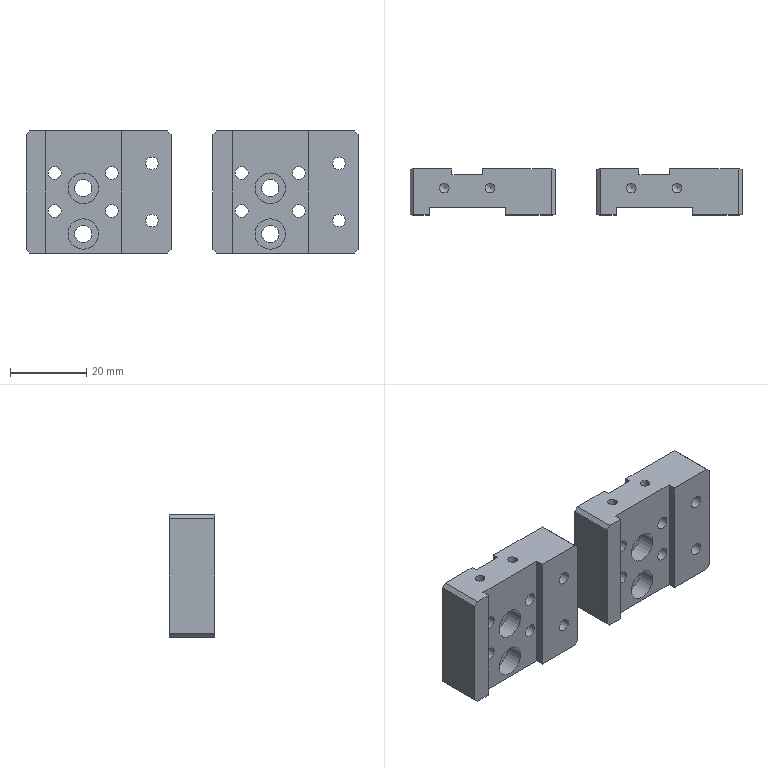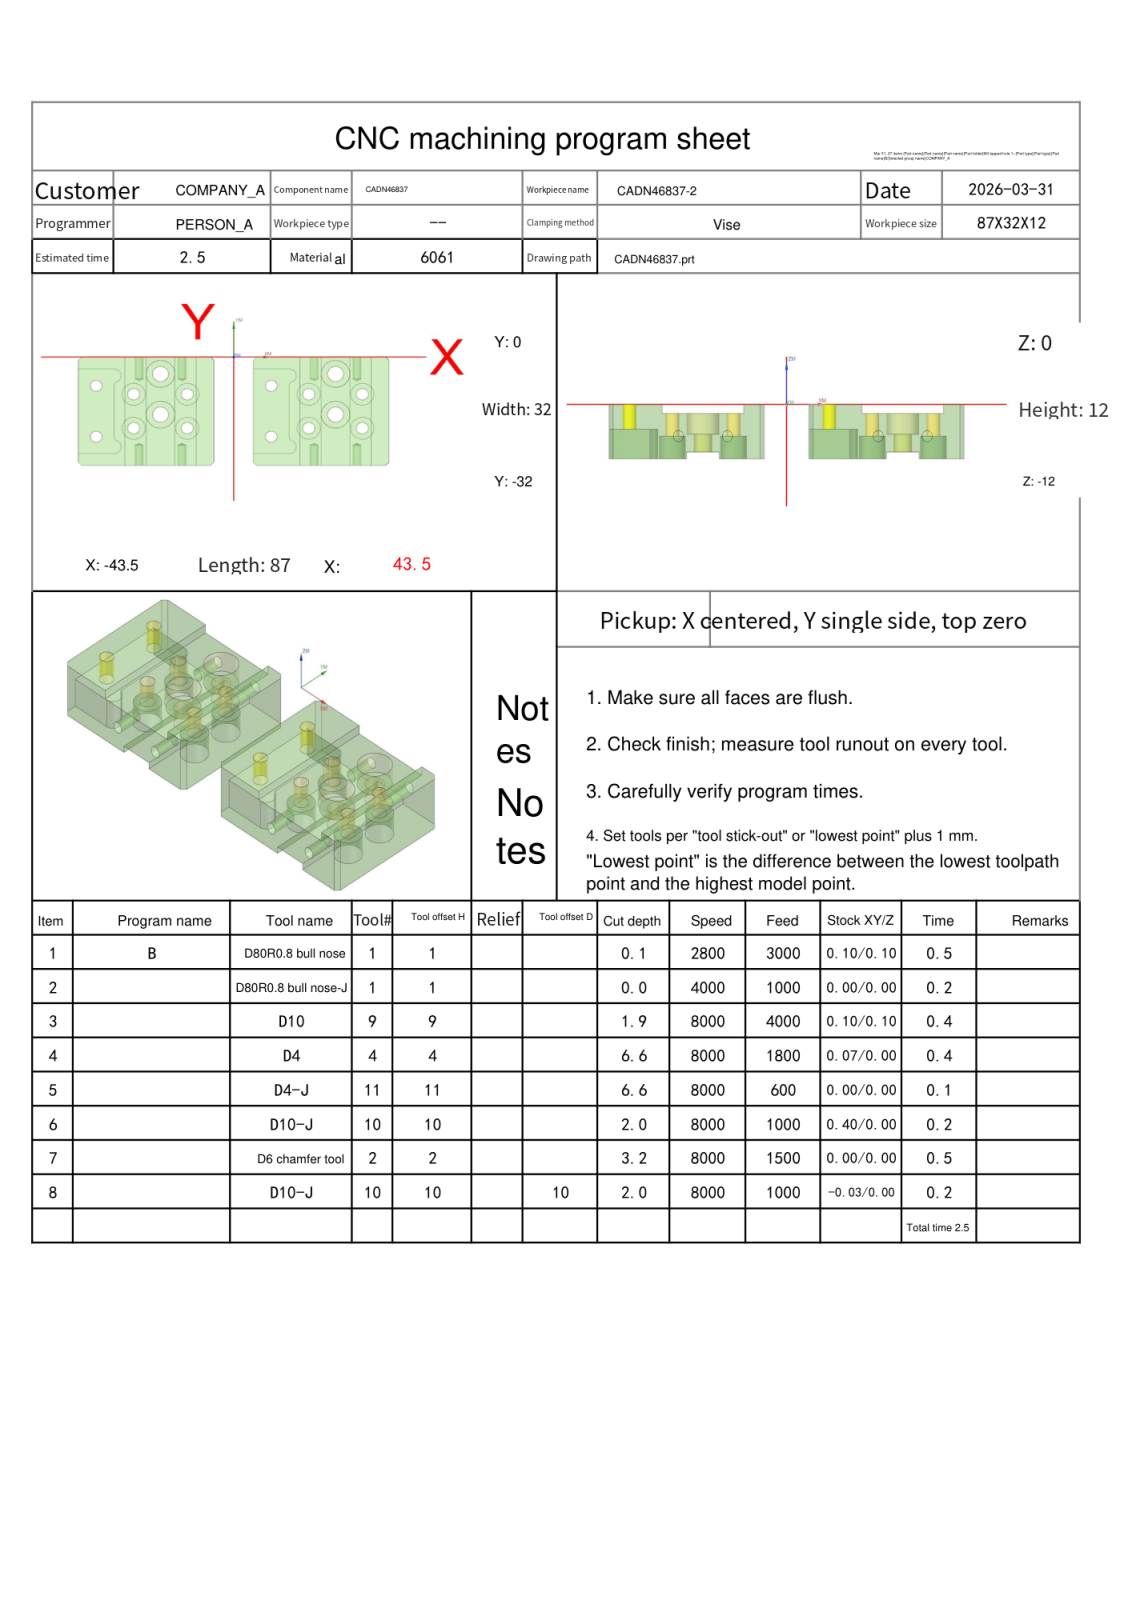NC program | NX | posted by the shop | part box 87 x 12 x 32 mm
Whole program:
%
O0001
(Machine time: 4.13 MIN)
(===Total Tool:6===)
(T1=D80R0.8 bull nose D=80.  R=0.8  D-  H01 Z=0.    )
(T9=D10     D=10.  R=0.   D-  H09 Z=-1.9  )
(T4=D4      D=4.   R=0.   D-  H04 Z=-6.6  )
(T11=D4-J   D=4.   R=0.   D-  H11 Z=-6.6  )
(T10=D10-J  D=10.  R=0.   D-  H10 Z=-2.   )
(T2=D6 chamfer tool   D=6.   R=0.   D-  H02 Z=-3.2  )
G80 G90 G17 G49 G40
G91 G28 Z0
M01
N1 T01 M06
(D80R0.8 bull nose  D=80. R=0.8 H=01 ce=0.10 di=0.10)
G00 G90 G54 X-95.597 Y-16. M03 S2800
G43 H01 Z20.
M08
Z4.517
G01 Z2.517 F3000.
X-83.597
X83.597
X95.597
Z4.517
G00 X-95.597
Z4.033
G01 Z2.033
X-83.597
X83.597
X95.597
Z4.033
G00 X-95.597
Z3.55
G01 Z1.55
X-83.597
X83.597
X95.597
Z3.55
G00 X-95.597
Z3.067
G01 Z1.067
X-83.597
X83.597
X95.597
Z3.067
G00 Z20.
X-95.597
Z2.583
G01 Z.583
X-83.597
X83.597
X95.597
Z2.583
G00 Z20.
X-95.597
Z2.1
G01 Z.1
X-83.597
X83.597
X95.597
Z2.1
G00 Z20.
G91 G28 Z0.0
M05
M09
G91 G28 Z0.0
M01
N2 T01 M06
(D80R0.8 bull nose-J  D=80. R=0.8 H=01 ce=0.00 di=0.00)
G00 G90 G54 X-95.499 Y-16. M03 S4000
G43 H01 Z20.
M08
Z2.
G01 Z0.0 F1000.
X-83.499
X83.499
X95.499
Z2.
G00 Z20.
G91 G28 Z0.0
M05
M09
G91 G28 Z0.0
M01
N3 T09 M06
(D10  D=10. R=0. H=09 ce=0.10 di=0.10)
G00 G90 G54 X-20.5 Y-40. M03 S8000
G43 H09 Z12.8
M08
Z1.025
G01 Z-.475 F4000.
Y-36.9
X-25.4
Y4.9
X-15.6
Y-36.9
X-17.632
G02 X-18.526 Y-36.347 I0.0 J1.
G01 X-20.324 Y-32.754
G03 X-20.705 Y-32.344 I-.894 J-.448
G02 X-20.9 Y-32.001 I.205 J.344
G01 Y.001
G02 X-20.5 Y.4 I.4 J-.001
X-20.1 Y.001 I0.0 J-.4
G01 Y-32.001
G02 X-20.5 Y-32.4 I-.4 J.001
G01 X-20.501
G02 X-20.88 Y-32.126 I.001 J.4
G01 X-23.727 Y-33.072
Y-40.1
Z1.025
G00 X-20.5 Y-40.
Z.55
G01 Z-.95
Y-36.9
X-25.4
Y4.9
X-15.6
Y-36.9
X-17.632
G02 X-18.526 Y-36.347 I0.0 J1.
G01 X-20.324 Y-32.754
G03 X-20.705 Y-32.344 I-.894 J-.448
G02 X-20.9 Y-32.001 I.205 J.344
G01 Y.001
G02 X-20.5 Y.4 I.4 J-.001
X-20.1 Y.001 I0.0 J-.4
G01 Y-32.001
G02 X-20.5 Y-32.4 I-.4 J.001
G01 X-20.501
G02 X-20.88 Y-32.126 I.001 J.4
G01 X-23.727 Y-33.072
Y-40.1
Z.55
G00 X-20.5 Y-40.
Z.075
G01 Z-1.425
Y-36.9
X-25.4
Y4.9
X-15.6
Y-36.9
X-17.632
G02 X-18.526 Y-36.347 I0.0 J1.
G01 X-20.324 Y-32.754
G03 X-20.705 Y-32.344 I-.894 J-.448
G02 X-20.9 Y-32.001 I.205 J.344
G01 Y.001
G02 X-20.5 Y.4 I.4 J-.001
X-20.1 Y.001 I0.0 J-.4
G01 Y-32.001
G02 X-20.5 Y-32.4 I-.4 J.001
G01 X-20.501
G02 X-20.88 Y-32.126 I.001 J.4
G01 X-23.727 Y-33.072
Y-40.1
Z.075
G00 X-20.5 Y-40.
Z-.4
G01 Z-1.9
Y-36.9
X-25.4
Y4.9
X-15.6
Y-36.9
X-17.632
G02 X-18.526 Y-36.347 I0.0 J1.
G01 X-20.324 Y-32.754
G03 X-20.705 Y-32.344 I-.894 J-.448
G02 X-20.9 Y-32.001 I.205 J.344
G01 Y.001
G02 X-20.5 Y.4 I.4 J-.001
X-20.1 Y.001 I0.0 J-.4
G01 Y-32.001
G02 X-20.5 Y-32.4 I-.4 J.001
G01 X-20.501
G02 X-20.88 Y-32.126 I.001 J.4
G01 X-23.727 Y-33.072
Y-40.1
Z-.4
G00 Z3.
X28.5 Y-40.
Z1.025
G01 Z-.475
Y-36.9
X23.6
Y4.9
X33.4
Y-36.9
X31.368
G02 X30.474 Y-36.347 I0.0 J1.
G01 X28.676 Y-32.754
G03 X28.295 Y-32.344 I-.894 J-.448
G02 X28.1 Y-32.001 I.205 J.344
G01 Y.001
G02 X28.5 Y.4 I.4 J-.001
X28.9 Y.001 I0.0 J-.4
G01 Y-32.001
G02 X28.5 Y-32.4 I-.4 J.001
X28.12 Y-32.126 I.001 J.4
G01 X25.273 Y-33.072
Y-40.1
Z1.025
G00 X28.5 Y-40.
Z.55
G01 Z-.95
Y-36.9
X23.6
Y4.9
X33.4
Y-36.9
X31.368
G02 X30.474 Y-36.347 I0.0 J1.
G01 X28.676 Y-32.754
G03 X28.295 Y-32.344 I-.894 J-.448
G02 X28.1 Y-32.001 I.205 J.344
G01 Y.001
G02 X28.5 Y.4 I.4 J-.001
X28.9 Y.001 I0.0 J-.4
G01 Y-32.001
G02 X28.5 Y-32.4 I-.4 J.001
X28.12 Y-32.126 I.001 J.4
G01 X25.273 Y-33.072
Y-40.1
Z.55
G00 X28.5 Y-40.
Z.075
G01 Z-1.425
Y-36.9
X23.6
Y4.9
X33.4
Y-36.9
X31.368
G02 X30.474 Y-36.347 I0.0 J1.
G01 X28.676 Y-32.754
G03 X28.295 Y-32.344 I-.894 J-.448
G02 X28.1 Y-32.001 I.205 J.344
G01 Y.001
G02 X28.5 Y.4 I.4 J-.001
X28.9 Y.001 I0.0 J-.4
G01 Y-32.001
G02 X28.5 Y-32.4 I-.4 J.001
X28.12 Y-32.126 I.001 J.4
G01 X25.273 Y-33.072
Y-40.1
Z.075
G00 X28.5 Y-40.
Z-.4
G01 Z-1.9
Y-36.9
X23.6
Y4.9
X33.4
Y-36.9
X31.368
G02 X30.474 Y-36.347 I0.0 J1.
G01 X28.676 Y-32.754
G03 X28.295 Y-32.344 I-.894 J-.448
G02 X28.1 Y-32.001 I.205 J.344
G01 Y.001
G02 X28.5 Y.4 I.4 J-.001
X28.9 Y.001 I0.0 J-.4
G01 Y-32.001
G02 X28.5 Y-32.4 I-.4 J.001
X28.12 Y-32.126 I.001 J.4
G01 X25.273 Y-33.072
Y-40.1
Z-.4
G00 Z12.8
G91 G28 Z0.0
M05
M09
G91 G28 Z0.0
M01
N4 T04 M06
(D4  D=4. R=0. H=04 ce=0.07 di=0.00)
G00 G90 G54 X-20.5 Y-17. M03 S8000
G43 H04 Z20.
M08
Z-1.7
G03 X-21.465 Y-16.035 I-.965 J0.0 F1800.
X-22.43 Y-17. I0.0 J-.965
X-22.43 Y-17. Z-2.05 I1.93 J0.0
X-22.43 Y-17. Z-2.4 I1.93 J0.0
X-22.43 Y-17. Z-2.75 I1.93 J0.0
X-22.43 Y-17. Z-3.1 I1.93 J0.0
X-22.43 Y-17. Z-3.45 I1.93 J0.0
X-22.43 Y-17. Z-3.8 I1.93 J0.0
X-22.43 Y-17. Z-4.15 I1.93 J0.0
X-22.43 Y-17. Z-4.5 I1.93 J0.0
X-22.43 Y-17. Z-4.85 I1.93 J0.0
X-22.43 Y-17. Z-5.2 I1.93 J0.0
X-22.43 Y-17. Z-5.55 I1.93 J0.0
X-22.43 Y-17. Z-5.9 I1.93 J0.0
X-22.43 Y-17. Z-6.25 I1.93 J0.0
X-22.43 Y-17. Z-6.6 I1.93 J0.0
X-20.5 Y-18.93 I1.93 J0.0
X-18.57 Y-17. I0.0 J1.93
X-20.5 Y-15.07 I-1.93 J0.0
X-22.43 Y-17. I0.0 J-1.93
X-21.465 Y-17.965 I.965 J0.0
X-20.5 Y-17. I0.0 J.965
G00 Z20.
Y-5.
Z-1.7
G03 X-21.465 Y-4.035 I-.965 J0.0
X-22.43 Y-5. I0.0 J-.965
X-22.43 Y-5. Z-2.05 I1.93 J0.0
X-22.43 Y-5. Z-2.4 I1.93 J0.0
X-22.43 Y-5. Z-2.75 I1.93 J0.0
X-22.43 Y-5. Z-3.1 I1.93 J0.0
X-22.43 Y-5. Z-3.45 I1.93 J0.0
X-22.43 Y-5. Z-3.8 I1.93 J0.0
X-22.43 Y-5. Z-4.15 I1.93 J0.0
X-22.43 Y-5. Z-4.5 I1.93 J0.0
X-22.43 Y-5. Z-4.85 I1.93 J0.0
X-22.43 Y-5. Z-5.2 I1.93 J0.0
X-22.43 Y-5. Z-5.55 I1.93 J0.0
X-22.43 Y-5. Z-5.9 I1.93 J0.0
X-22.43 Y-5. Z-6.25 I1.93 J0.0
X-22.43 Y-5. Z-6.6 I1.93 J0.0
X-20.5 Y-6.93 I1.93 J0.0
X-18.57 Y-5. I0.0 J1.93
X-20.5 Y-3.07 I-1.93 J0.0
X-22.43 Y-5. I0.0 J-1.93
X-21.465 Y-5.965 I.965 J0.0
X-20.5 Y-5. I0.0 J.965
G00 Z20.
X28.5
Z-1.7
G03 X27.535 Y-4.035 I-.965 J0.0
X26.57 Y-5. I0.0 J-.965
X26.57 Y-5. Z-2.05 I1.93 J0.0
X26.57 Y-5. Z-2.4 I1.93 J0.0
X26.57 Y-5. Z-2.75 I1.93 J0.0
X26.57 Y-5. Z-3.1 I1.93 J0.0
X26.57 Y-5. Z-3.45 I1.93 J0.0
X26.57 Y-5. Z-3.8 I1.93 J0.0
X26.57 Y-5. Z-4.15 I1.93 J0.0
X26.57 Y-5. Z-4.5 I1.93 J0.0
X26.57 Y-5. Z-4.85 I1.93 J0.0
X26.57 Y-5. Z-5.2 I1.93 J0.0
X26.57 Y-5. Z-5.55 I1.93 J0.0
X26.57 Y-5. Z-5.9 I1.93 J0.0
X26.57 Y-5. Z-6.25 I1.93 J0.0
X26.57 Y-5. Z-6.6 I1.93 J0.0
X28.5 Y-6.93 I1.93 J0.0
X30.43 Y-5. I0.0 J1.93
X28.5 Y-3.07 I-1.93 J0.0
X26.57 Y-5. I0.0 J-1.93
X27.535 Y-5.965 I.965 J0.0
X28.5 Y-5. I0.0 J.965
G00 Z20.
Y-17.
Z-1.7
G03 X27.535 Y-16.035 I-.965 J0.0
X26.57 Y-17. I0.0 J-.965
X26.57 Y-17. Z-2.05 I1.93 J0.0
X26.57 Y-17. Z-2.4 I1.93 J0.0
X26.57 Y-17. Z-2.75 I1.93 J0.0
X26.57 Y-17. Z-3.1 I1.93 J0.0
X26.57 Y-17. Z-3.45 I1.93 J0.0
X26.57 Y-17. Z-3.8 I1.93 J0.0
X26.57 Y-17. Z-4.15 I1.93 J0.0
X26.57 Y-17. Z-4.5 I1.93 J0.0
X26.57 Y-17. Z-4.85 I1.93 J0.0
X26.57 Y-17. Z-5.2 I1.93 J0.0
X26.57 Y-17. Z-5.55 I1.93 J0.0
X26.57 Y-17. Z-5.9 I1.93 J0.0
X26.57 Y-17. Z-6.25 I1.93 J0.0
X26.57 Y-17. Z-6.6 I1.93 J0.0
X28.5 Y-18.93 I1.93 J0.0
X30.43 Y-17. I0.0 J1.93
X28.5 Y-15.07 I-1.93 J0.0
X26.57 Y-17. I0.0 J-1.93
X27.535 Y-17.965 I.965 J0.0
X28.5 Y-17. I0.0 J.965
G00 Z20.
G91 G28 Z0.0
M05
M09
G91 G28 Z0.0
M01
N5 T11 M06
(D4-J  D=4. R=0. H=11 ce=0.00 di=0.00)
G00 G90 G54 X-20.5 Y-17. M03 S8000
G43 H11 Z20.
M08
Z-6.6
G01 X-22.096 Y-16.671 F600.
X-22.164 Y-16.664
G03 X-22.5 Y-17. I0.0 J-.336
X-20.5 Y-19. I2. J0.0
X-18.5 Y-17. I0.0 J2.
X-20.5 Y-15. I-2. J0.0
X-22.5 Y-17. I0.0 J-2.
X-22.438 Y-17.495 I2. J0.0
X-22.112 Y-17.748 I.325 J.083
G01 X-21.965 Y-17.714
X-20.5 Y-17.
G00 Z20.
Y-5.
Z-6.6
G01 X-22.096 Y-4.671
X-22.164 Y-4.664
G03 X-22.5 Y-5. I0.0 J-.336
X-20.5 Y-7. I2. J0.0
X-18.5 Y-5. I0.0 J2.
X-20.5 Y-3. I-2. J0.0
X-22.5 Y-5. I0.0 J-2.
X-22.438 Y-5.495 I2. J0.0
X-22.112 Y-5.748 I.325 J.083
G01 X-21.965 Y-5.714
X-20.5 Y-5.
G00 Z20.
X28.5
Z-6.6
G01 X26.904 Y-4.671
X26.836 Y-4.664
G03 X26.5 Y-5. I0.0 J-.336
X28.5 Y-7. I2. J0.0
X30.5 Y-5. I0.0 J2.
X28.5 Y-3. I-2. J0.0
X26.5 Y-5. I0.0 J-2.
X26.562 Y-5.495 I2. J0.0
X26.888 Y-5.748 I.325 J.083
G01 X27.035 Y-5.714
X28.5 Y-5.
G00 Z20.
Y-17.
Z-6.6
G01 X26.904 Y-16.671
X26.836 Y-16.664
G03 X26.5 Y-17. I0.0 J-.336
X28.5 Y-19. I2. J0.0
X30.5 Y-17. I0.0 J2.
X28.5 Y-15. I-2. J0.0
X26.5 Y-17. I0.0 J-2.
X26.562 Y-17.495 I2. J0.0
X26.888 Y-17.748 I.325 J.083
G01 X27.035 Y-17.714
X28.5 Y-17.
G00 Z20.
G91 G28 Z0.0
M05
M09
G91 G28 Z0.0
M01
N6 T10 M06
(D10-J  D=10. R=0. H=10 ce=0.40 di=0.00)
G00 G90 G54 X-22.5 Y7. M03 S8000
G43 H10 Z12.8
M08
Z-.5
G01 Z-2. F1000.
Y3.
G03 X-20.5 Y1. I2. J0.0
G01 X-16.898
G02 X-15.9 Y.002 I-.002 J-1.
G01 Y-32.002
G02 X-16.898 Y-33. I-1. J.002
G01 X-24.102
G02 X-25.1 Y-32.002 I.002 J1.
G01 Y.002
G02 X-24.102 Y1. I1. J-.002
G01 X-20.5
X-19.5
G03 X-17.5 Y3. I0.0 J2.
G01 Y7.4
Z-.5
G00 Z2.
X26.5 Y7.
Z-.5
G01 Z-2.
Y3.
G03 X28.5 Y1. I2. J0.0
G01 X32.102
G02 X33.1 Y.002 I-.002 J-1.
G01 Y-32.002
G02 X32.102 Y-33. I-1. J.002
G01 X24.898
G02 X23.9 Y-32.002 I.002 J1.
G01 Y.002
G02 X24.898 Y1. I1. J-.002
G01 X28.5
X29.5
G03 X31.5 Y3. I0.0 J2.
G01 Y7.4
Z-.5
G00 Z12.8
G91 G28 Z0.0
M05
M09
G91 G28 Z0.0
M01
N7 T02 M06
(D6 chamfer tool  D=6. R=0. H=02 ce=0.00 di=0.00)
G00 G90 G54 X-38.5 Y-8.5 M03 S8000
G43 H02 Z20.
M08
G98 G81 X-38.5 Y-8.5 Z-2.2 R3. F1000.
Y-23.5
X10.5
Y-8.5
G80
G00 Z20.
G00 G90 X37.273 Y-16.386 M03 S6500
Z20.
Z.172
G01 Z-1.2 F1500.
G03 X37.473 Y-16.1 I-1.532 J1.286
G01 X37.503 Y-16.054
X37.5 Y-16.
Y0.0
G02 X38.5 Y1. I1. J0.0
G01 X42.5
X42.759 Y.966
X43. Y.866
X43.207 Y.707
X44.207 Y-.293
X44.366 Y-.5
X44.466 Y-.741
X44.5 Y-1.
Y-31.
X44.466 Y-31.259
X44.366 Y-31.5
X44.207 Y-31.707
X43.207 Y-32.707
X43. Y-32.866
X42.759 Y-32.966
X42.5 Y-33.
X38.5
G02 X37.5 Y-32. I0.0 J1.
G01 Y-16.
X37.503 Y-15.946
X37.473 Y-15.9
G03 X37.273 Y-15.614 I-1.732 J-1.
G01 Z.172
G00 Z10.
X4.273 Y-16.386
Z.172
G01 Z-1.2
G03 X4.473 Y-16.1 I-1.532 J1.286
G01 X4.503 Y-16.054
X4.5 Y-16.
Y-1.
X4.534 Y-.741
X4.634 Y-.5
X4.793 Y-.293
X5.793 Y.707
X6. Y.866
X6.241 Y.966
X6.5 Y1.
X18.5
G02 X19.5 Y0.0 I0.0 J-1.
G01 Y-32.
G02 X18.5 Y-33. I-1. J0.0
G01 X6.5
X6.241 Y-32.966
X6. Y-32.866
X5.793 Y-32.707
X4.793 Y-31.707
X4.634 Y-31.5
X4.534 Y-31.259
X4.5 Y-31.
Y-16.
X4.503 Y-15.946
X4.473 Y-15.9
G03 X4.273 Y-15.614 I-1.732 J-1.
G01 Z.172
G00 Z2.55
X10.081 Y-8.994
Z.405
G01 Z-1.2
G03 X10.397 Y-9.141 I1. J1.732
G01 X10.447 Y-9.162
X10.5 Y-9.15
G03 X11.15 Y-8.5 I0.0 J.65
X10.5 Y-7.85 I-.65 J0.0
X9.85 Y-8.5 I0.0 J-.65
X10.5 Y-9.15 I.65 J0.0
G01 X10.553 Y-9.162
X10.603 Y-9.141
G03 X10.919 Y-8.994 I-.684 J1.879
G01 Z.405
G00 Z10.
X10.081 Y-23.994
Z.405
G01 Z-1.2
G03 X10.397 Y-24.141 I1. J1.732
G01 X10.447 Y-24.162
X10.5 Y-24.15
G03 X11.15 Y-23.5 I0.0 J.65
X10.5 Y-22.85 I-.65 J0.0
X9.85 Y-23.5 I0.0 J-.65
X10.5 Y-24.15 I.65 J0.0
G01 X10.553 Y-24.162
X10.603 Y-24.141
G03 X10.919 Y-23.994 I-.684 J1.879
G01 Z.405
G00 Z10.
X-11.727 Y-16.386
Z.172
G01 Z-1.2
G03 X-11.527 Y-16.1 I-1.532 J1.286
G01 X-11.497 Y-16.054
X-11.5 Y-16.
Y0.0
G02 X-10.5 Y1. I1. J0.0
G01 X-6.5
X-6.241 Y.966
X-6. Y.866
X-5.793 Y.707
X-4.793 Y-.293
X-4.634 Y-.5
X-4.534 Y-.741
X-4.5 Y-1.
Y-31.
X-4.534 Y-31.259
X-4.634 Y-31.5
X-4.793 Y-31.707
X-5.793 Y-32.707
X-6. Y-32.866
X-6.241 Y-32.966
X-6.5 Y-33.
X-10.5
G02 X-11.5 Y-32. I0.0 J1.
G01 Y-16.
X-11.497 Y-15.946
X-11.527 Y-15.9
G03 X-11.727 Y-15.614 I-1.732 J-1.
G01 Z.172
G00 Z10.
X-29.273
Z.172
G01 Z-1.2
G03 X-29.473 Y-15.9 I1.532 J-1.286
G01 X-29.503 Y-15.946
X-29.5 Y-16.
Y-32.
G02 X-30.5 Y-33. I-1. J0.0
G01 X-42.5
X-42.759 Y-32.966
X-43. Y-32.866
X-43.207 Y-32.707
X-44.207 Y-31.707
X-44.366 Y-31.5
X-44.466 Y-31.259
X-44.5 Y-31.
Y-1.
X-44.466 Y-.741
X-44.366 Y-.5
X-44.207 Y-.293
X-43.207 Y.707
X-43. Y.866
X-42.759 Y.966
X-42.5 Y1.
X-30.5
G02 X-29.5 Y0.0 I0.0 J-1.
G01 Y-16.
X-29.503 Y-16.054
X-29.473 Y-16.1
G03 X-29.273 Y-16.386 I1.732 J1.
G01 Z.172
G00 Z10.
X-38.919 Y-8.994
Z.405
G01 Z-1.2
G03 X-38.603 Y-9.141 I1. J1.732
G01 X-38.553 Y-9.162
X-38.5 Y-9.15
G03 X-37.85 Y-8.5 I0.0 J.65
X-38.5 Y-7.85 I-.65 J0.0
X-39.15 Y-8.5 I0.0 J-.65
X-38.5 Y-9.15 I.65 J0.0
G01 X-38.447 Y-9.162
X-38.397 Y-9.141
G03 X-38.081 Y-8.994 I-.684 J1.879
G01 Z.405
G00 Z10.
X-38.919 Y-23.994
Z.405
G01 Z-1.2
G03 X-38.603 Y-24.141 I1. J1.732
G01 X-38.553 Y-24.162
X-38.5 Y-24.15
G03 X-37.85 Y-23.5 I0.0 J.65
X-38.5 Y-22.85 I-.65 J0.0
X-39.15 Y-23.5 I0.0 J-.65
X-38.5 Y-24.15 I.65 J0.0
G01 X-38.447 Y-24.162
X-38.397 Y-24.141
G03 X-38.081 Y-23.994 I-.684 J1.879
G01 Z.405
G00 Z10.
X-27.53 Y1.068
Z-1.669
G01 Z-3.199
X-27.444 Y1.008
X-27.414 Y1.
X-13.586
X-13.556 Y1.008
X-13.47 Y1.068
Z-1.669
G00 Z10.
Y-33.068
Z-1.669
G01 Z-3.199
X-13.556 Y-33.008
X-13.586 Y-33.
X-27.414
X-27.444 Y-33.008
X-27.53 Y-33.068
Z-1.669
G00 Z10.
X-20.099 Y-2.197
Z-1.767
G01 Z-3.199
G03 X-20.398 Y-2.019 I-1.167 J-1.624
G01 X-20.446 Y-1.993
X-20.5 Y-2.
G03 X-23.5 Y-5. I0.0 J-3.
X-20.5 Y-8. I3. J0.0
X-17.5 Y-5. I0.0 J3.
X-20.5 Y-2. I-3. J0.0
G01 X-20.554 Y-1.993
X-20.602 Y-2.019
G03 X-20.901 Y-2.197 I.868 J-1.802
G01 Z-1.767
G00 Z10.
X-20.099 Y-14.197
Z-1.767
G01 Z-3.199
G03 X-20.398 Y-14.019 I-1.167 J-1.624
G01 X-20.446 Y-13.993
X-20.5 Y-14.
G03 X-23.5 Y-17. I0.0 J-3.
X-20.5 Y-20. I3. J0.0
X-17.5 Y-17. I0.0 J3.
X-20.5 Y-14. I-3. J0.0
G01 X-20.554 Y-13.993
X-20.602 Y-14.019
G03 X-20.901 Y-14.197 I.868 J-1.802
G01 Z-1.767
G00 Z10.
X21.47 Y1.068
Z-1.669
G01 Z-3.199
X21.556 Y1.008
X21.586 Y1.
X35.414
X35.444 Y1.008
X35.53 Y1.068
Z-1.669
G00 Z10.
Y-33.068
Z-1.669
G01 Z-3.199
X35.444 Y-33.008
X35.414 Y-33.
X21.586
X21.556 Y-33.008
X21.47 Y-33.068
Z-1.669
G00 Z10.
X28.901 Y-2.197
Z-1.767
G01 Z-3.199
G03 X28.602 Y-2.019 I-1.167 J-1.624
G01 X28.554 Y-1.993
X28.5 Y-2.
G03 X25.5 Y-5. I0.0 J-3.
X28.5 Y-8. I3. J0.0
X31.5 Y-5. I0.0 J3.
X28.5 Y-2. I-3. J0.0
G01 X28.446 Y-1.993
X28.398 Y-2.019
G03 X28.099 Y-2.197 I.868 J-1.802
G01 Z-1.767
G00 Z10.
X28.901 Y-14.197
Z-1.767
G01 Z-3.199
G03 X28.602 Y-14.019 I-1.167 J-1.624
G01 X28.554 Y-13.993
X28.5 Y-14.
G03 X25.5 Y-17. I0.0 J-3.
X28.5 Y-20. I3. J0.0
X31.5 Y-17. I0.0 J3.
X28.5 Y-14. I-3. J0.0
G01 X28.446 Y-13.993
X28.398 Y-14.019
G03 X28.099 Y-14.197 I.868 J-1.802
G01 Z-1.767
G00 Z20.
G91 G28 Z0.0
M05
M09
G91 G28 Z0.0
M01
N8 T10 M06
(D10-J  D=10. R=0. H=10 ce=-0.03 di=0.00)
G00 G90 G54 X-23.678 Y7.005 M03 S8000
G43 H10 Z12.8
M08
Z-1.
G01 Z-2. F1000.
G41 D10
X-23.875 Y6.97
G03 X-25.53 Y5. I.345 J-1.97
G01 Y-37.
G03 X-23.875 Y-38.97 I2. J0.0
G01 G40 X-23.678 Y-39.005
X-17.322
G41 D10
X-17.125 Y-38.97
G03 X-15.47 Y-37. I-.345 J1.97
G01 Y5.
G03 X-17.125 Y6.97 I-2. J0.0
G01 G40 X-17.322 Y7.005
Z-1.
G00 Z3.
X25.322
Z-1.
G01 Z-2.
G41 D10
X25.125 Y6.97
G03 X23.47 Y5. I.345 J-1.97
G01 Y-37.
G03 X25.125 Y-38.97 I2. J0.0
G01 G40 X25.322 Y-39.005
X31.678
G41 D10
X31.875 Y-38.97
G03 X33.53 Y-37. I-.345 J1.97
G01 Y5.
G03 X31.875 Y6.97 I-2. J0.0
G01 G40 X31.678 Y7.005
Z-1.
G00 Z12.8
M05
M09
G91 G28 Z0.0
G91 G28 Y0.0
M30
%